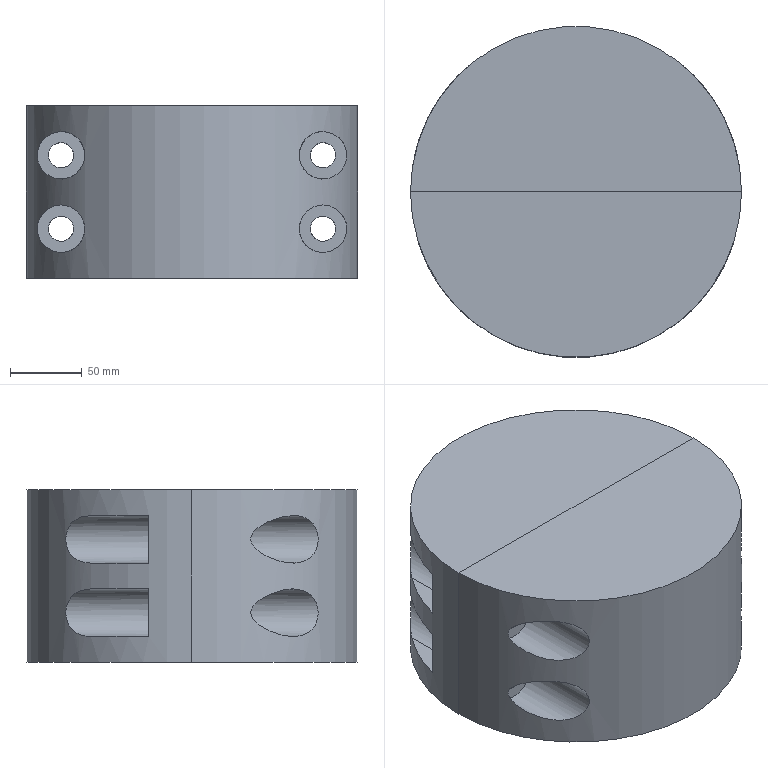NC program | NX | posted with a generic post | part box 230 x 230 x 120 mm
Whole program:
N10 G17 G21 G94 G90
(DRILLING_COPY_1_1 , TOOL : ZXZ)
N12 T02 M6
N14 G54
N16 G17 G0 G90 X-91. Y25.5 S3500 M3
N18 G43 Z30. H2
N20 G94 G81 G98 Z-1. F250. R3.
N22 Y-25.5
N24 X91.
N26 Y25.5
N28 G80
N30 G0 X91. Y25.5 Z30.
N32 M5
(DRILLING_COPY_COPY , TOOL : 17.5ZT)
N34 T04 M6
N36 G54
N38 G17 G0 G90 X-91. Y25.5 S500 M3
N40 G43 Z30. H4
N42 G94 G83 G98 Z-40.258 F80. Q3. R3.
N44 Y-25.5
N46 X91.
N48 Y25.5
N50 G80
N52 G0 X91. Y25.5 Z30.
N54 M5
(THREAD_MILLING , TOOL : D15XYD)
N56 T05 M6
N58 G54
N60 G17 G0 G90 X-91. Y-25.5 S1200 M3
N62 G43 Z30. H5
N64 Z0.964
N66 G42 G94 G1 X-91.517 Y-24.957 F500. D5
N68 G2 X-90.305 Y-23.36 Z0.5 R1.061
N70 X-90.305 Y-23.36 Z-2. I-0.695 J-2.14
N72 X-90.305 Y-23.36 Z-4.5 I-0.695 J-2.14
N74 X-90.305 Y-23.36 Z-7. I-0.695 J-2.14
N76 X-90.305 Y-23.36 Z-9.5 I-0.695 J-2.14
N78 X-90.305 Y-23.36 Z-12. I-0.695 J-2.14
N80 X-90.305 Y-23.36 Z-14.5 I-0.695 J-2.14
N82 X-90.305 Y-23.36 Z-17. I-0.695 J-2.14
N84 X-90.305 Y-23.36 Z-19.5 I-0.695 J-2.14
N86 X-90.305 Y-23.36 Z-22. I-0.695 J-2.14
N88 X-90.305 Y-23.36 Z-24.5 I-0.695 J-2.14
N90 X-90.305 Y-23.36 Z-27. I-0.695 J-2.14
N92 X-90.305 Y-23.36 Z-29.5 I-0.695 J-2.14
N94 X-88.75 Y-25.5 Z-30. R2.25
N96 X-90.643 Y-26.16 Z-30.464 R1.061
N98 G40
N100 G1 X-91. Y-25.5
N102 G0 Z1.001
N104 G42 G1 X-91.579 Y-25.023
N106 G2 X-90.15 Y-22.885 Z0.5 R1.336
N108 X-90.15 Y-22.885 Z-2. I-0.85 J-2.615
N110 X-90.15 Y-22.885 Z-4.5 I-0.85 J-2.615
N112 X-90.15 Y-22.885 Z-7. I-0.85 J-2.615
N114 X-90.15 Y-22.885 Z-9.5 I-0.85 J-2.615
N116 X-90.15 Y-22.885 Z-12. I-0.85 J-2.615
N118 X-90.15 Y-22.885 Z-14.5 I-0.85 J-2.615
N120 X-90.15 Y-22.885 Z-17. I-0.85 J-2.615
N122 X-90.15 Y-22.885 Z-19.5 I-0.85 J-2.615
N124 X-90.15 Y-22.885 Z-22. I-0.85 J-2.615
N126 X-90.15 Y-22.885 Z-24.5 I-0.85 J-2.615
N128 X-90.15 Y-22.885 Z-27. I-0.85 J-2.615
N130 X-90.15 Y-22.885 Z-29.5 I-0.85 J-2.615
N132 X-88.25 Y-25.5 Z-30. R2.75
N134 X-90.725 Y-26.198 Z-30.501 R1.336
N136 G40
N138 G1 X-91. Y-25.5
N140 G0 Z1.025
N142 G42 G1 X-91.617 Y-25.074
N144 G2 X-89.996 Y-22.409 Z0.5 R1.603
N146 X-89.996 Y-22.409 Z-2. I-1.004 J-3.091
N148 X-89.996 Y-22.409 Z-4.5 I-1.004 J-3.091
N150 X-89.996 Y-22.409 Z-7. I-1.004 J-3.091
N152 X-89.996 Y-22.409 Z-9.5 I-1.004 J-3.091
N154 X-89.996 Y-22.409 Z-12. I-1.004 J-3.091
N156 X-89.996 Y-22.409 Z-14.5 I-1.004 J-3.091
N158 X-89.996 Y-22.409 Z-17. I-1.004 J-3.091
N160 X-89.996 Y-22.409 Z-19.5 I-1.004 J-3.091
N162 X-89.996 Y-22.409 Z-22. I-1.004 J-3.091
N164 X-89.996 Y-22.409 Z-24.5 I-1.004 J-3.091
N166 X-89.996 Y-22.409 Z-27. I-1.004 J-3.091
N168 X-89.996 Y-22.409 Z-29.5 I-1.004 J-3.091
N170 X-87.75 Y-25.5 Z-30. R3.25
N172 X-90.785 Y-26.219 Z-30.525 R1.603
N174 G40
N176 G1 X-91. Y-25.5
N178 G0 Z30.
N180 Y25.5
N182 Z0.964
N184 G42 G1 X-91.517 Y26.043
N186 G2 X-90.305 Y27.64 Z0.5 R1.061
N188 X-90.305 Y27.64 Z-2. I-0.695 J-2.14
N190 X-90.305 Y27.64 Z-4.5 I-0.695 J-2.14
N192 X-90.305 Y27.64 Z-7. I-0.695 J-2.14
N194 X-90.305 Y27.64 Z-9.5 I-0.695 J-2.14
N196 X-90.305 Y27.64 Z-12. I-0.695 J-2.14
N198 X-90.305 Y27.64 Z-14.5 I-0.695 J-2.14
N200 X-90.305 Y27.64 Z-17. I-0.695 J-2.14
N202 X-90.305 Y27.64 Z-19.5 I-0.695 J-2.14
N204 X-90.305 Y27.64 Z-22. I-0.695 J-2.14
N206 X-90.305 Y27.64 Z-24.5 I-0.695 J-2.14
N208 X-90.305 Y27.64 Z-27. I-0.695 J-2.14
N210 X-90.305 Y27.64 Z-29.5 I-0.695 J-2.14
N212 X-88.75 Y25.5 Z-30. R2.25
N214 X-90.643 Y24.84 Z-30.464 R1.061
N216 G40
N218 G1 X-91. Y25.5
N220 G0 Z1.001
N222 G42 G1 X-91.579 Y25.977
N224 G2 X-90.15 Y28.115 Z0.5 R1.336
N226 X-90.15 Y28.115 Z-2. I-0.85 J-2.615
N228 X-90.15 Y28.115 Z-4.5 I-0.85 J-2.615
N230 X-90.15 Y28.115 Z-7. I-0.85 J-2.615
N232 X-90.15 Y28.115 Z-9.5 I-0.85 J-2.615
N234 X-90.15 Y28.115 Z-12. I-0.85 J-2.615
N236 X-90.15 Y28.115 Z-14.5 I-0.85 J-2.615
N238 X-90.15 Y28.115 Z-17. I-0.85 J-2.615
N240 X-90.15 Y28.115 Z-19.5 I-0.85 J-2.615
N242 X-90.15 Y28.115 Z-22. I-0.85 J-2.615
N244 X-90.15 Y28.115 Z-24.5 I-0.85 J-2.615
N246 X-90.15 Y28.115 Z-27. I-0.85 J-2.615
N248 X-90.15 Y28.115 Z-29.5 I-0.85 J-2.615
N250 X-88.25 Y25.5 Z-30. R2.75
N252 X-90.725 Y24.802 Z-30.501 R1.336
N254 G40
N256 G1 X-91. Y25.5
N258 G0 Z1.025
N260 G42 G1 X-91.617 Y25.926
N262 G2 X-89.996 Y28.591 Z0.5 R1.603
N264 X-89.996 Y28.591 Z-2. I-1.004 J-3.091
N266 X-89.996 Y28.591 Z-4.5 I-1.004 J-3.091
N268 X-89.996 Y28.591 Z-7. I-1.004 J-3.091
N270 X-89.996 Y28.591 Z-9.5 I-1.004 J-3.091
N272 X-89.996 Y28.591 Z-12. I-1.004 J-3.091
N274 X-89.996 Y28.591 Z-14.5 I-1.004 J-3.091
N276 X-89.996 Y28.591 Z-17. I-1.004 J-3.091
N278 X-89.996 Y28.591 Z-19.5 I-1.004 J-3.091
N280 X-89.996 Y28.591 Z-22. I-1.004 J-3.091
N282 X-89.996 Y28.591 Z-24.5 I-1.004 J-3.091
N284 X-89.996 Y28.591 Z-27. I-1.004 J-3.091
N286 X-89.996 Y28.591 Z-29.5 I-1.004 J-3.091
N288 X-87.75 Y25.5 Z-30. R3.25
N290 X-90.785 Y24.781 Z-30.525 R1.603
N292 G40
N294 G1 X-91. Y25.5
N296 G0 Z30.
N298 X91.
N300 Z0.964
N302 G42 G1 X90.483 Y26.043
N304 G2 X91.695 Y27.64 Z0.5 R1.061
N306 X91.695 Y27.64 Z-2. I-0.695 J-2.14
N308 X91.695 Y27.64 Z-4.5 I-0.695 J-2.14
N310 X91.695 Y27.64 Z-7. I-0.695 J-2.14
N312 X91.695 Y27.64 Z-9.5 I-0.695 J-2.14
N314 X91.695 Y27.64 Z-12. I-0.695 J-2.14
N316 X91.695 Y27.64 Z-14.5 I-0.695 J-2.14
N318 X91.695 Y27.64 Z-17. I-0.695 J-2.14
N320 X91.695 Y27.64 Z-19.5 I-0.695 J-2.14
N322 X91.695 Y27.64 Z-22. I-0.695 J-2.14
N324 X91.695 Y27.64 Z-24.5 I-0.695 J-2.14
N326 X91.695 Y27.64 Z-27. I-0.695 J-2.14
N328 X91.695 Y27.64 Z-29.5 I-0.695 J-2.14
N330 X93.25 Y25.5 Z-30. R2.25
N332 X91.357 Y24.84 Z-30.464 R1.061
N334 G40
N336 G1 X91. Y25.5
N338 G0 Z1.001
N340 G42 G1 X90.421 Y25.977
N342 G2 X91.85 Y28.115 Z0.5 R1.336
N344 X91.85 Y28.115 Z-2. I-0.85 J-2.615
N346 X91.85 Y28.115 Z-4.5 I-0.85 J-2.615
N348 X91.85 Y28.115 Z-7. I-0.85 J-2.615
N350 X91.85 Y28.115 Z-9.5 I-0.85 J-2.615
N352 X91.85 Y28.115 Z-12. I-0.85 J-2.615
N354 X91.85 Y28.115 Z-14.5 I-0.85 J-2.615
N356 X91.85 Y28.115 Z-17. I-0.85 J-2.615
N358 X91.85 Y28.115 Z-19.5 I-0.85 J-2.615
N360 X91.85 Y28.115 Z-22. I-0.85 J-2.615
N362 X91.85 Y28.115 Z-24.5 I-0.85 J-2.615
N364 X91.85 Y28.115 Z-27. I-0.85 J-2.615
N366 X91.85 Y28.115 Z-29.5 I-0.85 J-2.615
N368 X93.75 Y25.5 Z-30. R2.75
N370 X91.275 Y24.802 Z-30.501 R1.336
N372 G40
N374 G1 X91. Y25.5
N376 G0 Z1.025
N378 G42 G1 X90.383 Y25.926
N380 G2 X92.004 Y28.591 Z0.5 R1.603
N382 X92.004 Y28.591 Z-2. I-1.004 J-3.091
N384 X92.004 Y28.591 Z-4.5 I-1.004 J-3.091
N386 X92.004 Y28.591 Z-7. I-1.004 J-3.091
N388 X92.004 Y28.591 Z-9.5 I-1.004 J-3.091
N390 X92.004 Y28.591 Z-12. I-1.004 J-3.091
N392 X92.004 Y28.591 Z-14.5 I-1.004 J-3.091
N394 X92.004 Y28.591 Z-17. I-1.004 J-3.091
N396 X92.004 Y28.591 Z-19.5 I-1.004 J-3.091
N398 X92.004 Y28.591 Z-22. I-1.004 J-3.091
N400 X92.004 Y28.591 Z-24.5 I-1.004 J-3.091
N402 X92.004 Y28.591 Z-27. I-1.004 J-3.091
N404 X92.004 Y28.591 Z-29.5 I-1.004 J-3.091
N406 X94.25 Y25.5 Z-30. R3.25
N408 X91.215 Y24.781 Z-30.525 R1.603
N410 G40
N412 G1 X91. Y25.5
N414 G0 Z30.
N416 Y-25.5
N418 Z0.964
N420 G42 G1 X90.483 Y-24.957
N422 G2 X91.695 Y-23.36 Z0.5 R1.061
N424 X91.695 Y-23.36 Z-2. I-0.695 J-2.14
N426 X91.695 Y-23.36 Z-4.5 I-0.695 J-2.14
N428 X91.695 Y-23.36 Z-7. I-0.695 J-2.14
N430 X91.695 Y-23.36 Z-9.5 I-0.695 J-2.14
N432 X91.695 Y-23.36 Z-12. I-0.695 J-2.14
N434 X91.695 Y-23.36 Z-14.5 I-0.695 J-2.14
N436 X91.695 Y-23.36 Z-17. I-0.695 J-2.14
N438 X91.695 Y-23.36 Z-19.5 I-0.695 J-2.14
N440 X91.695 Y-23.36 Z-22. I-0.695 J-2.14
N442 X91.695 Y-23.36 Z-24.5 I-0.695 J-2.14
N444 X91.695 Y-23.36 Z-27. I-0.695 J-2.14
N446 X91.695 Y-23.36 Z-29.5 I-0.695 J-2.14
N448 X93.25 Y-25.5 Z-30. R2.25
N450 X91.357 Y-26.16 Z-30.464 R1.061
N452 G40
N454 G1 X91. Y-25.5
N456 G0 Z1.001
N458 G42 G1 X90.421 Y-25.023
N460 G2 X91.85 Y-22.885 Z0.5 R1.336
N462 X91.85 Y-22.885 Z-2. I-0.85 J-2.615
N464 X91.85 Y-22.885 Z-4.5 I-0.85 J-2.615
N466 X91.85 Y-22.885 Z-7. I-0.85 J-2.615
N468 X91.85 Y-22.885 Z-9.5 I-0.85 J-2.615
N470 X91.85 Y-22.885 Z-12. I-0.85 J-2.615
N472 X91.85 Y-22.885 Z-14.5 I-0.85 J-2.615
N474 X91.85 Y-22.885 Z-17. I-0.85 J-2.615
N476 X91.85 Y-22.885 Z-19.5 I-0.85 J-2.615
N478 X91.85 Y-22.885 Z-22. I-0.85 J-2.615
N480 X91.85 Y-22.885 Z-24.5 I-0.85 J-2.615
N482 X91.85 Y-22.885 Z-27. I-0.85 J-2.615
N484 X91.85 Y-22.885 Z-29.5 I-0.85 J-2.615
N486 X93.75 Y-25.5 Z-30. R2.75
N488 X91.275 Y-26.198 Z-30.501 R1.336
N490 G40
N492 G1 X91. Y-25.5
N494 G0 Z1.025
N496 G42 G1 X90.383 Y-25.074
N498 G2 X92.004 Y-22.409 Z0.5 R1.603
N500 X92.004 Y-22.409 Z-2. I-1.004 J-3.091
N502 X92.004 Y-22.409 Z-4.5 I-1.004 J-3.091
N504 X92.004 Y-22.409 Z-7. I-1.004 J-3.091
N506 X92.004 Y-22.409 Z-9.5 I-1.004 J-3.091
N508 X92.004 Y-22.409 Z-12. I-1.004 J-3.091
N510 X92.004 Y-22.409 Z-14.5 I-1.004 J-3.091
N512 X92.004 Y-22.409 Z-17. I-1.004 J-3.091
N514 X92.004 Y-22.409 Z-19.5 I-1.004 J-3.091
N516 X92.004 Y-22.409 Z-22. I-1.004 J-3.091
N518 X92.004 Y-22.409 Z-24.5 I-1.004 J-3.091
N520 X92.004 Y-22.409 Z-27. I-1.004 J-3.091
N522 X92.004 Y-22.409 Z-29.5 I-1.004 J-3.091
N524 X94.25 Y-25.5 Z-30. R3.25
N526 X91.215 Y-26.219 Z-30.525 R1.603
N528 G40
N530 G1 X91. Y-25.5
N532 G0 Z30.
(THREAD_MILLING_COPY , TOOL : D15XYD)
N534 X-91.
N536 Z1.025
N538 G42 G1 X-91.617 Y-25.074
N540 G2 X-89.996 Y-22.409 Z0.5 R1.603
N542 X-89.996 Y-22.409 Z-2. I-1.004 J-3.091
N544 X-89.996 Y-22.409 Z-4.5 I-1.004 J-3.091
N546 X-89.996 Y-22.409 Z-7. I-1.004 J-3.091
N548 X-89.996 Y-22.409 Z-9.5 I-1.004 J-3.091
N550 X-89.996 Y-22.409 Z-12. I-1.004 J-3.091
N552 X-89.996 Y-22.409 Z-14.5 I-1.004 J-3.091
N554 X-89.996 Y-22.409 Z-17. I-1.004 J-3.091
N556 X-89.996 Y-22.409 Z-19.5 I-1.004 J-3.091
N558 X-89.996 Y-22.409 Z-22. I-1.004 J-3.091
N560 X-89.996 Y-22.409 Z-24.5 I-1.004 J-3.091
N562 X-89.996 Y-22.409 Z-27. I-1.004 J-3.091
N564 X-89.996 Y-22.409 Z-29.5 I-1.004 J-3.091
N566 X-87.75 Y-25.5 Z-30. R3.25
N568 X-90.785 Y-26.219 Z-30.525 R1.603
N570 G40
N572 G1 X-91. Y-25.5
N574 G0 Z30.
N576 Y25.5
N578 Z1.025
N580 G42 G1 X-91.617 Y25.926
N582 G2 X-89.996 Y28.591 Z0.5 R1.603
N584 X-89.996 Y28.591 Z-2. I-1.004 J-3.091
N586 X-89.996 Y28.591 Z-4.5 I-1.004 J-3.091
N588 X-89.996 Y28.591 Z-7. I-1.004 J-3.091
N590 X-89.996 Y28.591 Z-9.5 I-1.004 J-3.091
N592 X-89.996 Y28.591 Z-12. I-1.004 J-3.091
N594 X-89.996 Y28.591 Z-14.5 I-1.004 J-3.091
N596 X-89.996 Y28.591 Z-17. I-1.004 J-3.091
N598 X-89.996 Y28.591 Z-19.5 I-1.004 J-3.091
N600 X-89.996 Y28.591 Z-22. I-1.004 J-3.091
N602 X-89.996 Y28.591 Z-24.5 I-1.004 J-3.091
N604 X-89.996 Y28.591 Z-27. I-1.004 J-3.091
N606 X-89.996 Y28.591 Z-29.5 I-1.004 J-3.091
N608 X-87.75 Y25.5 Z-30. R3.25
N610 X-90.785 Y24.781 Z-30.525 R1.603
N612 G40
N614 G1 X-91. Y25.5
N616 G0 Z30.
N618 X91.
N620 Z1.025
N622 G42 G1 X90.383 Y25.926
N624 G2 X92.004 Y28.591 Z0.5 R1.603
N626 X92.004 Y28.591 Z-2. I-1.004 J-3.091
N628 X92.004 Y28.591 Z-4.5 I-1.004 J-3.091
N630 X92.004 Y28.591 Z-7. I-1.004 J-3.091
N632 X92.004 Y28.591 Z-9.5 I-1.004 J-3.091
N634 X92.004 Y28.591 Z-12. I-1.004 J-3.091
N636 X92.004 Y28.591 Z-14.5 I-1.004 J-3.091
N638 X92.004 Y28.591 Z-17. I-1.004 J-3.091
N640 X92.004 Y28.591 Z-19.5 I-1.004 J-3.091
N642 X92.004 Y28.591 Z-22. I-1.004 J-3.091
N644 X92.004 Y28.591 Z-24.5 I-1.004 J-3.091
N646 X92.004 Y28.591 Z-27. I-1.004 J-3.091
N648 X92.004 Y28.591 Z-29.5 I-1.004 J-3.091
N650 X94.25 Y25.5 Z-30. R3.25
N652 X91.215 Y24.781 Z-30.525 R1.603
N654 G40
N656 G1 X91. Y25.5
N658 G0 Z30.
N660 Y-25.5
N662 Z1.025
N664 G42 G1 X90.383 Y-25.074
N666 G2 X92.004 Y-22.409 Z0.5 R1.603
N668 X92.004 Y-22.409 Z-2. I-1.004 J-3.091
N670 X92.004 Y-22.409 Z-4.5 I-1.004 J-3.091
N672 X92.004 Y-22.409 Z-7. I-1.004 J-3.091
N674 X92.004 Y-22.409 Z-9.5 I-1.004 J-3.091
N676 X92.004 Y-22.409 Z-12. I-1.004 J-3.091
N678 X92.004 Y-22.409 Z-14.5 I-1.004 J-3.091
N680 X92.004 Y-22.409 Z-17. I-1.004 J-3.091
N682 X92.004 Y-22.409 Z-19.5 I-1.004 J-3.091
N684 X92.004 Y-22.409 Z-22. I-1.004 J-3.091
N686 X92.004 Y-22.409 Z-24.5 I-1.004 J-3.091
N688 X92.004 Y-22.409 Z-27. I-1.004 J-3.091
N690 X92.004 Y-22.409 Z-29.5 I-1.004 J-3.091
N692 X94.25 Y-25.5 Z-30. R3.25
N694 X91.215 Y-26.219 Z-30.525 R1.603
N696 G40
N698 G1 X91. Y-25.5
N700 G0 Z30.
N702 M5
N704 M2